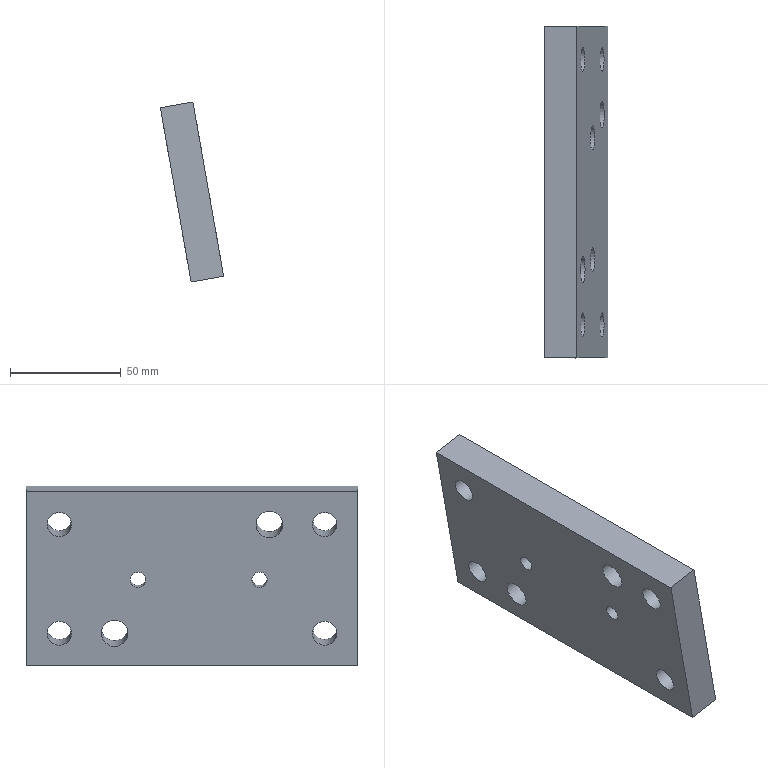Part | NX | features solid 2 | 1 solid | 18 faces | box 28.664 x 150 x 81.389 mm | volume 168620 mm3 | cylinder 10 | plane 8 | commonest cylinder face diameters 11 x6 7 x2 12 x2
STEP:
#1=CARTESIAN_POINT('',(748.926,-438.051,-1.716));
#2=VERTEX_POINT('',#1);
#3=CARTESIAN_POINT('',(735.034,-438.051,77.069));
#4=VERTEX_POINT('',#3);
#5=CARTESIAN_POINT('',(752.051,-438.051,-19.442));
#6=DIRECTION('',(-0.1736,0.000000436,0.9848));
#7=VECTOR('',#6,1000.);
#8=LINE('',#5,#7);
#9=EDGE_CURVE('',#2,#4,#8,.T.);
#10=ORIENTED_EDGE('',*,*,#9,.T.);
#11=CARTESIAN_POINT('',(749.806,-438.051,79.673));
#12=VERTEX_POINT('',#11);
#13=CARTESIAN_POINT('',(749.806,-438.051,79.673));
#14=DIRECTION('',(-0.9848,0.000001617,-0.1736));
#15=VECTOR('',#14,1000.);
#16=LINE('',#13,#15);
#17=EDGE_CURVE('',#12,#4,#16,.T.);
#18=ORIENTED_EDGE('',*,*,#17,.F.);
#19=CARTESIAN_POINT('',(763.698,-438.051,0.8888));
#20=VERTEX_POINT('',#19);
#21=CARTESIAN_POINT('',(766.823,-438.051,-16.838));
#22=DIRECTION('',(-0.1736,0.000000436,0.9848));
#23=VECTOR('',#22,1000.);
#24=LINE('',#21,#23);
#25=EDGE_CURVE('',#20,#12,#24,.T.);
#26=ORIENTED_EDGE('',*,*,#25,.F.);
#27=CARTESIAN_POINT('',(763.698,-438.051,0.8888));
#28=DIRECTION('',(-0.9848,0.000001617,-0.1736));
#29=VECTOR('',#28,1000.);
#30=LINE('',#27,#29);
#31=EDGE_CURVE('',#20,#2,#30,.T.);
#32=ORIENTED_EDGE('',*,*,#31,.T.);
#33=EDGE_LOOP('',(#10,#18,#26,#32));
#34=FACE_BOUND('',#33,.T.);
#35=CARTESIAN_POINT('',(766.823,-438.051,-16.838));
#36=DIRECTION('',(0.000001668,1.,-0.000000149));
#37=DIRECTION('',(1.,-0.000001668,0.));
#38=AXIS2_PLACEMENT_3D('',#35,#36,#37);
#39=PLANE('',#38);
#40=ADVANCED_FACE('',(#34),#39,.T.);
#41=CARTESIAN_POINT('',(735.033,-588.051,77.069));
#42=VERTEX_POINT('',#41);
#43=CARTESIAN_POINT('',(735.034,-438.051,77.069));
#44=DIRECTION('',(-0.000001668,-1.,0.000000149));
#45=VECTOR('',#44,1000.);
#46=LINE('',#43,#45);
#47=EDGE_CURVE('',#4,#42,#46,.T.);
#48=ORIENTED_EDGE('',*,*,#47,.T.);
#49=CARTESIAN_POINT('',(749.806,-588.051,79.673));
#50=VERTEX_POINT('',#49);
#51=CARTESIAN_POINT('',(749.806,-588.051,79.673));
#52=DIRECTION('',(-0.9848,0.000001617,-0.1736));
#53=VECTOR('',#52,1000.);
#54=LINE('',#51,#53);
#55=EDGE_CURVE('',#50,#42,#54,.T.);
#56=ORIENTED_EDGE('',*,*,#55,.F.);
#57=CARTESIAN_POINT('',(749.806,-438.051,79.673));
#58=DIRECTION('',(-0.000001668,-1.,0.000000149));
#59=VECTOR('',#58,1000.);
#60=LINE('',#57,#59);
#61=EDGE_CURVE('',#12,#50,#60,.T.);
#62=ORIENTED_EDGE('',*,*,#61,.F.);
#63=ORIENTED_EDGE('',*,*,#17,.T.);
#64=EDGE_LOOP('',(#48,#56,#62,#63));
#65=FACE_BOUND('',#64,.T.);
#66=CARTESIAN_POINT('',(749.806,-438.051,79.673));
#67=DIRECTION('',(-0.1736,0.000000436,0.9848));
#68=DIRECTION('',(-0.9848,0.,-0.1736));
#69=AXIS2_PLACEMENT_3D('',#66,#67,#68);
#70=PLANE('',#69);
#71=ADVANCED_FACE('',(#65),#70,.T.);
#72=CARTESIAN_POINT('',(748.925,-588.051,-1.716));
#73=VERTEX_POINT('',#72);
#74=CARTESIAN_POINT('',(752.051,-588.051,-19.442));
#75=DIRECTION('',(-0.1736,0.000000436,0.9848));
#76=VECTOR('',#75,1000.);
#77=LINE('',#74,#76);
#78=EDGE_CURVE('',#73,#42,#77,.T.);
#79=ORIENTED_EDGE('',*,*,#78,.F.);
#80=CARTESIAN_POINT('',(763.697,-588.051,0.8888));
#81=VERTEX_POINT('',#80);
#82=CARTESIAN_POINT('',(763.697,-588.051,0.8888));
#83=DIRECTION('',(-0.9848,0.000001617,-0.1736));
#84=VECTOR('',#83,1000.);
#85=LINE('',#82,#84);
#86=EDGE_CURVE('',#81,#73,#85,.T.);
#87=ORIENTED_EDGE('',*,*,#86,.F.);
#88=CARTESIAN_POINT('',(766.823,-588.051,-16.838));
#89=DIRECTION('',(-0.1736,0.000000436,0.9848));
#90=VECTOR('',#89,1000.);
#91=LINE('',#88,#90);
#92=EDGE_CURVE('',#81,#50,#91,.T.);
#93=ORIENTED_EDGE('',*,*,#92,.T.);
#94=ORIENTED_EDGE('',*,*,#55,.T.);
#95=EDGE_LOOP('',(#79,#87,#93,#94));
#96=FACE_BOUND('',#95,.T.);
#97=CARTESIAN_POINT('',(766.823,-588.051,-16.838));
#98=DIRECTION('',(0.000001668,1.,-0.000000149));
#99=DIRECTION('',(1.,-0.000001668,0.));
#100=AXIS2_PLACEMENT_3D('',#97,#98,#99);
#101=PLANE('',#100);
#102=ADVANCED_FACE('',(#96),#101,.F.);
#103=ORIENTED_EDGE('',*,*,#86,.T.);
#104=CARTESIAN_POINT('',(748.926,-438.051,-1.716));
#105=DIRECTION('',(0.000001667,1.,-0.00000014));
#106=VECTOR('',#105,1000.);
#107=LINE('',#104,#106);
#108=EDGE_CURVE('',#73,#2,#107,.T.);
#109=ORIENTED_EDGE('',*,*,#108,.T.);
#110=ORIENTED_EDGE('',*,*,#31,.F.);
#111=CARTESIAN_POINT('',(763.698,-520.051,0.8888));
#112=DIRECTION('',(-0.000001667,-1.,0.00000014));
#113=VECTOR('',#112,1000.);
#114=LINE('',#111,#113);
#115=EDGE_CURVE('',#20,#81,#114,.T.);
#116=ORIENTED_EDGE('',*,*,#115,.T.);
#117=EDGE_LOOP('',(#103,#109,#110,#116));
#118=FACE_BOUND('',#117,.T.);
#119=CARTESIAN_POINT('',(763.698,-520.051,0.8888));
#120=DIRECTION('',(0.1736,-0.000000427,-0.9848));
#121=DIRECTION('',(0.9848,0.,0.1736));
#122=AXIS2_PLACEMENT_3D('',#119,#120,#121);
#123=PLANE('',#122);
#124=ADVANCED_FACE('',(#118),#123,.T.);
#125=CARTESIAN_POINT('',(757.776,-543.593,34.473));
#126=VERTEX_POINT('',#125);
#127=CARTESIAN_POINT('',(756.821,-543.593,39.889));
#128=DIRECTION('',(0.9848,-0.000001617,0.1736));
#129=DIRECTION('',(0.1736,0.,-0.9848));
#130=AXIS2_PLACEMENT_3D('',#127,#128,#129);
#131=CIRCLE('',#130,5.5);
#132=EDGE_CURVE('',#126,#126,#131,.T.);
#133=ORIENTED_EDGE('',*,*,#132,.F.);
#134=EDGE_LOOP('',(#133));
#135=FACE_BOUND('',#134,.T.);
#136=CARTESIAN_POINT('',(757.776,-488.593,34.473));
#137=VERTEX_POINT('',#136);
#138=CARTESIAN_POINT('',(756.821,-488.593,39.889));
#139=DIRECTION('',(0.9848,-0.000001617,0.1736));
#140=DIRECTION('',(0.1736,0.,-0.9848));
#141=AXIS2_PLACEMENT_3D('',#138,#139,#140);
#142=CIRCLE('',#141,5.5);
#143=EDGE_CURVE('',#137,#137,#142,.T.);
#144=ORIENTED_EDGE('',*,*,#143,.F.);
#145=EDGE_LOOP('',(#144));
#146=FACE_BOUND('',#145,.T.);
#147=CARTESIAN_POINT('',(762.135,-478.051,9.752));
#148=VERTEX_POINT('',#147);
#149=CARTESIAN_POINT('',(761.093,-478.051,15.661));
#150=DIRECTION('',(0.9848,-0.000001617,0.1736));
#151=DIRECTION('',(0.1736,0.,-0.9848));
#152=AXIS2_PLACEMENT_3D('',#149,#150,#151);
#153=CIRCLE('',#152,6.);
#154=EDGE_CURVE('',#148,#148,#153,.T.);
#155=ORIENTED_EDGE('',*,*,#154,.F.);
#156=EDGE_LOOP('',(#155));
#157=FACE_BOUND('',#156,.T.);
#158=CARTESIAN_POINT('',(753.452,-548.051,58.992));
#159=VERTEX_POINT('',#158);
#160=CARTESIAN_POINT('',(752.41,-548.051,64.901));
#161=DIRECTION('',(0.9848,-0.000001617,0.1736));
#162=DIRECTION('',(0.1736,0.,-0.9848));
#163=AXIS2_PLACEMENT_3D('',#160,#161,#162);
#164=CIRCLE('',#163,6.);
#165=EDGE_CURVE('',#159,#159,#164,.T.);
#166=ORIENTED_EDGE('',*,*,#165,.F.);
#167=EDGE_LOOP('',(#166));
#168=FACE_BOUND('',#167,.T.);
#169=CARTESIAN_POINT('',(762.048,-453.051,10.244));
#170=VERTEX_POINT('',#169);
#171=CARTESIAN_POINT('',(761.093,-453.051,15.661));
#172=DIRECTION('',(0.9848,-0.000001617,0.1736));
#173=DIRECTION('',(0.1736,0.,-0.9848));
#174=AXIS2_PLACEMENT_3D('',#171,#172,#173);
#175=CIRCLE('',#174,5.5);
#176=EDGE_CURVE('',#170,#170,#175,.T.);
#177=ORIENTED_EDGE('',*,*,#176,.F.);
#178=EDGE_LOOP('',(#177));
#179=FACE_BOUND('',#178,.T.);
#180=CARTESIAN_POINT('',(753.366,-453.051,59.485));
#181=VERTEX_POINT('',#180);
#182=CARTESIAN_POINT('',(752.411,-453.051,64.901));
#183=DIRECTION('',(0.9848,-0.000001617,0.1736));
#184=DIRECTION('',(0.1736,0.,-0.9848));
#185=AXIS2_PLACEMENT_3D('',#182,#183,#184);
#186=CIRCLE('',#185,5.5);
#187=EDGE_CURVE('',#181,#181,#186,.T.);
#188=ORIENTED_EDGE('',*,*,#187,.F.);
#189=EDGE_LOOP('',(#188));
#190=FACE_BOUND('',#189,.T.);
#191=CARTESIAN_POINT('',(762.048,-573.051,10.244));
#192=VERTEX_POINT('',#191);
#193=CARTESIAN_POINT('',(761.093,-573.051,15.661));
#194=DIRECTION('',(0.9848,-0.000001617,0.1736));
#195=DIRECTION('',(0.1736,0.,-0.9848));
#196=AXIS2_PLACEMENT_3D('',#193,#194,#195);
#197=CIRCLE('',#196,5.5);
#198=EDGE_CURVE('',#192,#192,#197,.T.);
#199=ORIENTED_EDGE('',*,*,#198,.F.);
#200=EDGE_LOOP('',(#199));
#201=FACE_BOUND('',#200,.T.);
#202=CARTESIAN_POINT('',(753.365,-573.051,59.485));
#203=VERTEX_POINT('',#202);
#204=CARTESIAN_POINT('',(752.41,-573.051,64.901));
#205=DIRECTION('',(0.9848,-0.000001617,0.1736));
#206=DIRECTION('',(0.1736,0.,-0.9848));
#207=AXIS2_PLACEMENT_3D('',#204,#205,#206);
#208=CIRCLE('',#207,5.5);
#209=EDGE_CURVE('',#203,#203,#208,.T.);
#210=ORIENTED_EDGE('',*,*,#209,.F.);
#211=EDGE_LOOP('',(#210));
#212=FACE_BOUND('',#211,.T.);
#213=ORIENTED_EDGE('',*,*,#115,.F.);
#214=ORIENTED_EDGE('',*,*,#25,.T.);
#215=ORIENTED_EDGE('',*,*,#61,.T.);
#216=ORIENTED_EDGE('',*,*,#92,.F.);
#217=EDGE_LOOP('',(#213,#214,#215,#216));
#218=FACE_BOUND('',#217,.T.);
#219=CARTESIAN_POINT('',(766.823,-438.051,-16.838));
#220=DIRECTION('',(-0.9848,0.000001617,-0.1736));
#221=DIRECTION('',(-0.1736,0.000000436,0.9848));
#222=AXIS2_PLACEMENT_3D('',#219,#220,#221);
#223=PLANE('',#222);
#224=ADVANCED_FACE('',(#135,#146,#157,#168,#179,#190,#201,#212,#218),#223,.F.);
#225=CARTESIAN_POINT('',(742.656,-543.593,33.838));
#226=VERTEX_POINT('',#225);
#227=CARTESIAN_POINT('',(742.049,-543.593,37.284));
#228=DIRECTION('',(0.9848,-0.000001617,0.1736));
#229=DIRECTION('',(0.1736,0.,-0.9848));
#230=AXIS2_PLACEMENT_3D('',#227,#228,#229);
#231=CIRCLE('',#230,3.5);
#232=EDGE_CURVE('',#226,#226,#231,.T.);
#233=ORIENTED_EDGE('',*,*,#232,.T.);
#234=EDGE_LOOP('',(#233));
#235=FACE_BOUND('',#234,.T.);
#236=CARTESIAN_POINT('',(742.656,-488.593,33.838));
#237=VERTEX_POINT('',#236);
#238=CARTESIAN_POINT('',(742.049,-488.593,37.284));
#239=DIRECTION('',(0.9848,-0.000001617,0.1736));
#240=DIRECTION('',(0.1736,0.,-0.9848));
#241=AXIS2_PLACEMENT_3D('',#238,#239,#240);
#242=CIRCLE('',#241,3.5);
#243=EDGE_CURVE('',#237,#237,#242,.T.);
#244=ORIENTED_EDGE('',*,*,#243,.T.);
#245=EDGE_LOOP('',(#244));
#246=FACE_BOUND('',#245,.T.);
#247=CARTESIAN_POINT('',(747.363,-478.051,7.147));
#248=VERTEX_POINT('',#247);
#249=CARTESIAN_POINT('',(746.321,-478.051,13.056));
#250=DIRECTION('',(0.9848,-0.000001617,0.1736));
#251=DIRECTION('',(0.1736,0.,-0.9848));
#252=AXIS2_PLACEMENT_3D('',#249,#250,#251);
#253=CIRCLE('',#252,6.);
#254=EDGE_CURVE('',#248,#248,#253,.T.);
#255=ORIENTED_EDGE('',*,*,#254,.T.);
#256=EDGE_LOOP('',(#255));
#257=FACE_BOUND('',#256,.T.);
#258=CARTESIAN_POINT('',(738.68,-548.051,56.388));
#259=VERTEX_POINT('',#258);
#260=CARTESIAN_POINT('',(737.638,-548.051,62.297));
#261=DIRECTION('',(0.9848,-0.000001617,0.1736));
#262=DIRECTION('',(0.1736,0.,-0.9848));
#263=AXIS2_PLACEMENT_3D('',#260,#261,#262);
#264=CIRCLE('',#263,6.);
#265=EDGE_CURVE('',#259,#259,#264,.T.);
#266=ORIENTED_EDGE('',*,*,#265,.T.);
#267=EDGE_LOOP('',(#266));
#268=FACE_BOUND('',#267,.T.);
#269=CARTESIAN_POINT('',(747.276,-453.051,7.64));
#270=VERTEX_POINT('',#269);
#271=CARTESIAN_POINT('',(746.321,-453.051,13.056));
#272=DIRECTION('',(0.9848,-0.000001617,0.1736));
#273=DIRECTION('',(0.1736,0.,-0.9848));
#274=AXIS2_PLACEMENT_3D('',#271,#272,#273);
#275=CIRCLE('',#274,5.5);
#276=EDGE_CURVE('',#270,#270,#275,.T.);
#277=ORIENTED_EDGE('',*,*,#276,.T.);
#278=EDGE_LOOP('',(#277));
#279=FACE_BOUND('',#278,.T.);
#280=CARTESIAN_POINT('',(738.593,-453.051,56.88));
#281=VERTEX_POINT('',#280);
#282=CARTESIAN_POINT('',(737.638,-453.051,62.297));
#283=DIRECTION('',(0.9848,-0.000001617,0.1736));
#284=DIRECTION('',(0.1736,0.,-0.9848));
#285=AXIS2_PLACEMENT_3D('',#282,#283,#284);
#286=CIRCLE('',#285,5.5);
#287=EDGE_CURVE('',#281,#281,#286,.T.);
#288=ORIENTED_EDGE('',*,*,#287,.T.);
#289=EDGE_LOOP('',(#288));
#290=FACE_BOUND('',#289,.T.);
#291=CARTESIAN_POINT('',(747.276,-573.051,7.64));
#292=VERTEX_POINT('',#291);
#293=CARTESIAN_POINT('',(746.321,-573.051,13.056));
#294=DIRECTION('',(0.9848,-0.000001617,0.1736));
#295=DIRECTION('',(0.1736,0.,-0.9848));
#296=AXIS2_PLACEMENT_3D('',#293,#294,#295);
#297=CIRCLE('',#296,5.5);
#298=EDGE_CURVE('',#292,#292,#297,.T.);
#299=ORIENTED_EDGE('',*,*,#298,.T.);
#300=EDGE_LOOP('',(#299));
#301=FACE_BOUND('',#300,.T.);
#302=CARTESIAN_POINT('',(738.593,-573.051,56.88));
#303=VERTEX_POINT('',#302);
#304=CARTESIAN_POINT('',(737.638,-573.051,62.297));
#305=DIRECTION('',(0.9848,-0.000001617,0.1736));
#306=DIRECTION('',(0.1736,0.,-0.9848));
#307=AXIS2_PLACEMENT_3D('',#304,#305,#306);
#308=CIRCLE('',#307,5.5);
#309=EDGE_CURVE('',#303,#303,#308,.T.);
#310=ORIENTED_EDGE('',*,*,#309,.T.);
#311=EDGE_LOOP('',(#310));
#312=FACE_BOUND('',#311,.T.);
#313=ORIENTED_EDGE('',*,*,#108,.F.);
#314=ORIENTED_EDGE('',*,*,#78,.T.);
#315=ORIENTED_EDGE('',*,*,#47,.F.);
#316=ORIENTED_EDGE('',*,*,#9,.F.);
#317=EDGE_LOOP('',(#313,#314,#315,#316));
#318=FACE_BOUND('',#317,.T.);
#319=CARTESIAN_POINT('',(752.051,-438.051,-19.442));
#320=DIRECTION('',(-0.9848,0.000001617,-0.1736));
#321=DIRECTION('',(-0.1736,0.000000436,0.9848));
#322=AXIS2_PLACEMENT_3D('',#319,#320,#321);
#323=PLANE('',#322);
#324=ADVANCED_FACE('',(#235,#246,#257,#268,#279,#290,#301,#312,#318),#323,.T.);
#325=ORIENTED_EDGE('',*,*,#309,.F.);
#326=EDGE_LOOP('',(#325));
#327=FACE_BOUND('',#326,.T.);
#328=ORIENTED_EDGE('',*,*,#209,.T.);
#329=EDGE_LOOP('',(#328));
#330=FACE_BOUND('',#329,.T.);
#331=CARTESIAN_POINT('',(621.431,-573.051,41.806));
#332=DIRECTION('',(0.9848,-0.000001617,0.1736));
#333=DIRECTION('',(-0.1736,0.,0.9848));
#334=AXIS2_PLACEMENT_3D('',#331,#332,#333);
#335=CYLINDRICAL_SURFACE('',#334,5.5);
#336=ADVANCED_FACE('',(#327,#330),#335,.F.);
#337=ORIENTED_EDGE('',*,*,#298,.F.);
#338=EDGE_LOOP('',(#337));
#339=FACE_BOUND('',#338,.T.);
#340=ORIENTED_EDGE('',*,*,#198,.T.);
#341=EDGE_LOOP('',(#340));
#342=FACE_BOUND('',#341,.T.);
#343=CARTESIAN_POINT('',(630.113,-573.051,-7.434));
#344=DIRECTION('',(0.9848,-0.000001617,0.1736));
#345=DIRECTION('',(-0.1736,0.,0.9848));
#346=AXIS2_PLACEMENT_3D('',#343,#344,#345);
#347=CYLINDRICAL_SURFACE('',#346,5.5);
#348=ADVANCED_FACE('',(#339,#342),#347,.F.);
#349=ORIENTED_EDGE('',*,*,#287,.F.);
#350=EDGE_LOOP('',(#349));
#351=FACE_BOUND('',#350,.T.);
#352=ORIENTED_EDGE('',*,*,#187,.T.);
#353=EDGE_LOOP('',(#352));
#354=FACE_BOUND('',#353,.T.);
#355=CARTESIAN_POINT('',(621.431,-453.051,41.806));
#356=DIRECTION('',(0.9848,-0.000001617,0.1736));
#357=DIRECTION('',(-0.1736,0.,0.9848));
#358=AXIS2_PLACEMENT_3D('',#355,#356,#357);
#359=CYLINDRICAL_SURFACE('',#358,5.5);
#360=ADVANCED_FACE('',(#351,#354),#359,.F.);
#361=ORIENTED_EDGE('',*,*,#276,.F.);
#362=EDGE_LOOP('',(#361));
#363=FACE_BOUND('',#362,.T.);
#364=ORIENTED_EDGE('',*,*,#176,.T.);
#365=EDGE_LOOP('',(#364));
#366=FACE_BOUND('',#365,.T.);
#367=CARTESIAN_POINT('',(630.113,-453.051,-7.434));
#368=DIRECTION('',(0.9848,-0.000001617,0.1736));
#369=DIRECTION('',(-0.1736,0.,0.9848));
#370=AXIS2_PLACEMENT_3D('',#367,#368,#369);
#371=CYLINDRICAL_SURFACE('',#370,5.5);
#372=ADVANCED_FACE('',(#363,#366),#371,.F.);
#373=ORIENTED_EDGE('',*,*,#265,.F.);
#374=EDGE_LOOP('',(#373));
#375=FACE_BOUND('',#374,.T.);
#376=ORIENTED_EDGE('',*,*,#165,.T.);
#377=EDGE_LOOP('',(#376));
#378=FACE_BOUND('',#377,.T.);
#379=CARTESIAN_POINT('',(836.119,-548.051,79.661));
#380=DIRECTION('',(-0.9848,0.000001617,-0.1736));
#381=DIRECTION('',(0.1736,0.,-0.9848));
#382=AXIS2_PLACEMENT_3D('',#379,#380,#381);
#383=CYLINDRICAL_SURFACE('',#382,6.);
#384=ADVANCED_FACE('',(#375,#378),#383,.F.);
#385=ORIENTED_EDGE('',*,*,#254,.F.);
#386=EDGE_LOOP('',(#385));
#387=FACE_BOUND('',#386,.T.);
#388=ORIENTED_EDGE('',*,*,#154,.T.);
#389=EDGE_LOOP('',(#388));
#390=FACE_BOUND('',#389,.T.);
#391=CARTESIAN_POINT('',(844.802,-478.052,30.421));
#392=DIRECTION('',(-0.9848,0.000001617,-0.1736));
#393=DIRECTION('',(0.1736,0.,-0.9848));
#394=AXIS2_PLACEMENT_3D('',#391,#392,#393);
#395=CYLINDRICAL_SURFACE('',#394,6.);
#396=ADVANCED_FACE('',(#387,#390),#395,.F.);
#397=CARTESIAN_POINT('',(747.928,-488.593,32.736));
#398=VERTEX_POINT('',#397);
#399=CARTESIAN_POINT('',(746.973,-488.593,38.153));
#400=DIRECTION('',(0.9848,-0.000001617,0.1736));
#401=DIRECTION('',(0.1736,0.,-0.9848));
#402=AXIS2_PLACEMENT_3D('',#399,#400,#401);
#403=CIRCLE('',#402,5.5);
#404=EDGE_CURVE('',#398,#398,#403,.F.);
#405=ORIENTED_EDGE('',*,*,#404,.T.);
#406=EDGE_LOOP('',(#405));
#407=FACE_BOUND('',#406,.T.);
#408=ORIENTED_EDGE('',*,*,#143,.T.);
#409=EDGE_LOOP('',(#408));
#410=FACE_BOUND('',#409,.T.);
#411=CARTESIAN_POINT('',(751.897,-488.593,39.021));
#412=DIRECTION('',(0.9848,-0.000001617,0.1736));
#413=DIRECTION('',(-0.1736,0.,0.9848));
#414=AXIS2_PLACEMENT_3D('',#411,#412,#413);
#415=CYLINDRICAL_SURFACE('',#414,5.5);
#416=ADVANCED_FACE('',(#407,#410),#415,.F.);
#417=ORIENTED_EDGE('',*,*,#243,.F.);
#418=EDGE_LOOP('',(#417));
#419=FACE_BOUND('',#418,.T.);
#420=CARTESIAN_POINT('',(747.58,-488.593,34.706));
#421=VERTEX_POINT('',#420);
#422=CARTESIAN_POINT('',(746.973,-488.593,38.153));
#423=DIRECTION('',(0.9848,-0.000001617,0.1736));
#424=DIRECTION('',(0.1736,0.,-0.9848));
#425=AXIS2_PLACEMENT_3D('',#422,#423,#424);
#426=CIRCLE('',#425,3.5);
#427=EDGE_CURVE('',#421,#421,#426,.F.);
#428=ORIENTED_EDGE('',*,*,#427,.F.);
#429=EDGE_LOOP('',(#428));
#430=FACE_BOUND('',#429,.T.);
#431=CARTESIAN_POINT('',(732.201,-488.593,35.548));
#432=DIRECTION('',(0.9848,-0.000001617,0.1736));
#433=DIRECTION('',(-0.1736,0.,0.9848));
#434=AXIS2_PLACEMENT_3D('',#431,#432,#433);
#435=CYLINDRICAL_SURFACE('',#434,3.5);
#436=ADVANCED_FACE('',(#419,#430),#435,.F.);
#437=ORIENTED_EDGE('',*,*,#427,.T.);
#438=EDGE_LOOP('',(#437));
#439=FACE_BOUND('',#438,.T.);
#440=ORIENTED_EDGE('',*,*,#404,.F.);
#441=EDGE_LOOP('',(#440));
#442=FACE_BOUND('',#441,.T.);
#443=CARTESIAN_POINT('',(746.973,-488.593,38.153));
#444=DIRECTION('',(-0.9848,0.000001617,-0.1736));
#445=DIRECTION('',(0.1736,0.,-0.9848));
#446=AXIS2_PLACEMENT_3D('',#443,#444,#445);
#447=PLANE('',#446);
#448=ADVANCED_FACE('',(#439,#442),#447,.F.);
#449=CARTESIAN_POINT('',(747.928,-543.593,32.736));
#450=VERTEX_POINT('',#449);
#451=CARTESIAN_POINT('',(746.973,-543.593,38.153));
#452=DIRECTION('',(0.9848,-0.000001617,0.1736));
#453=DIRECTION('',(0.1736,0.,-0.9848));
#454=AXIS2_PLACEMENT_3D('',#451,#452,#453);
#455=CIRCLE('',#454,5.5);
#456=EDGE_CURVE('',#450,#450,#455,.F.);
#457=ORIENTED_EDGE('',*,*,#456,.T.);
#458=EDGE_LOOP('',(#457));
#459=FACE_BOUND('',#458,.T.);
#460=ORIENTED_EDGE('',*,*,#132,.T.);
#461=EDGE_LOOP('',(#460));
#462=FACE_BOUND('',#461,.T.);
#463=CARTESIAN_POINT('',(751.897,-543.593,39.021));
#464=DIRECTION('',(0.9848,-0.000001617,0.1736));
#465=DIRECTION('',(-0.1736,0.,0.9848));
#466=AXIS2_PLACEMENT_3D('',#463,#464,#465);
#467=CYLINDRICAL_SURFACE('',#466,5.5);
#468=ADVANCED_FACE('',(#459,#462),#467,.F.);
#469=ORIENTED_EDGE('',*,*,#232,.F.);
#470=EDGE_LOOP('',(#469));
#471=FACE_BOUND('',#470,.T.);
#472=CARTESIAN_POINT('',(747.58,-543.593,34.706));
#473=VERTEX_POINT('',#472);
#474=CARTESIAN_POINT('',(746.973,-543.593,38.153));
#475=DIRECTION('',(0.9848,-0.000001617,0.1736));
#476=DIRECTION('',(0.1736,0.,-0.9848));
#477=AXIS2_PLACEMENT_3D('',#474,#475,#476);
#478=CIRCLE('',#477,3.5);
#479=EDGE_CURVE('',#473,#473,#478,.F.);
#480=ORIENTED_EDGE('',*,*,#479,.F.);
#481=EDGE_LOOP('',(#480));
#482=FACE_BOUND('',#481,.T.);
#483=CARTESIAN_POINT('',(732.201,-543.593,35.548));
#484=DIRECTION('',(0.9848,-0.000001617,0.1736));
#485=DIRECTION('',(-0.1736,0.,0.9848));
#486=AXIS2_PLACEMENT_3D('',#483,#484,#485);
#487=CYLINDRICAL_SURFACE('',#486,3.5);
#488=ADVANCED_FACE('',(#471,#482),#487,.F.);
#489=ORIENTED_EDGE('',*,*,#479,.T.);
#490=EDGE_LOOP('',(#489));
#491=FACE_BOUND('',#490,.T.);
#492=ORIENTED_EDGE('',*,*,#456,.F.);
#493=EDGE_LOOP('',(#492));
#494=FACE_BOUND('',#493,.T.);
#495=CARTESIAN_POINT('',(746.973,-543.593,38.153));
#496=DIRECTION('',(-0.9848,0.000001617,-0.1736));
#497=DIRECTION('',(0.1736,0.,-0.9848));
#498=AXIS2_PLACEMENT_3D('',#495,#496,#497);
#499=PLANE('',#498);
#500=ADVANCED_FACE('',(#491,#494),#499,.F.);
#501=CLOSED_SHELL('',(#40,#71,#102,#124,#224,#324,#336,#348,#360,#372,#384,#396,#416,#436,#448,#468,#488,#500));
#502=MANIFOLD_SOLID_BREP('',#501);
#503=(LENGTH_UNIT()NAMED_UNIT(*)SI_UNIT(.MILLI.,.METRE.));
#504=UNCERTAINTY_MEASURE_WITH_UNIT(LENGTH_MEASURE(0.00001),#503,'','');
#505=(NAMED_UNIT(*)PLANE_ANGLE_UNIT()SI_UNIT($,.RADIAN.));
#506=(NAMED_UNIT(*)SI_UNIT($,.STERADIAN.)SOLID_ANGLE_UNIT());
#507=(GEOMETRIC_REPRESENTATION_CONTEXT(3)GLOBAL_UNCERTAINTY_ASSIGNED_CONTEXT((#504))GLOBAL_UNIT_ASSIGNED_CONTEXT((#503,#505,#506))REPRESENTATION_CONTEXT('',''));
#508=ADVANCED_BREP_SHAPE_REPRESENTATION('',(#502),#507);